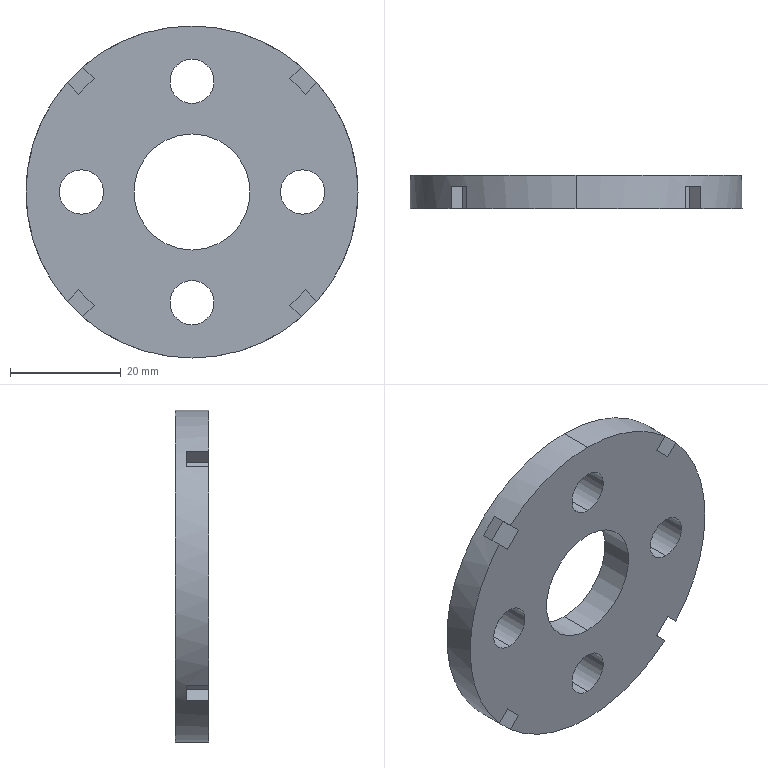Part | STEP file | Guide wheel mechanism revised.sldasm-Part-426 | 1 solid | 30 faces | box 60 x 6 x 60 mm | volume 13489 mm3 | plane 18 | cylinder 12 | commonest cylinder face diameters 8 x8 21 x2 60 x2
STEP:
#1=CARTESIAN_POINT('',(-20.,0.,4.));
#2=VERTEX_POINT('',#1);
#3=CARTESIAN_POINT('',(-20.,0.,-4.));
#4=VERTEX_POINT('',#3);
#5=CARTESIAN_POINT('',(-20.,0.,0.));
#6=DIRECTION('',(0.,-1.,0.));
#7=DIRECTION('',(0.,0.,1.));
#8=AXIS2_PLACEMENT_3D('',#5,#6,#7);
#9=CIRCLE('',#8,4.);
#10=EDGE_CURVE('',#2,#4,#9,.T.);
#11=ORIENTED_EDGE('',*,*,#10,.T.);
#12=CARTESIAN_POINT('',(-20.,6.,-4.));
#13=VERTEX_POINT('',#12);
#14=CARTESIAN_POINT('',(-20.,-0.001,-4.));
#15=DIRECTION('',(0.,1.,0.));
#16=VECTOR('',#15,1000.);
#17=LINE('',#14,#16);
#18=EDGE_CURVE('',#4,#13,#17,.T.);
#19=ORIENTED_EDGE('',*,*,#18,.T.);
#20=CARTESIAN_POINT('',(-20.,6.,4.));
#21=VERTEX_POINT('',#20);
#22=CARTESIAN_POINT('',(-20.,6.,0.));
#23=DIRECTION('',(0.,1.,0.));
#24=DIRECTION('',(0.,0.,1.));
#25=AXIS2_PLACEMENT_3D('',#22,#23,#24);
#26=CIRCLE('',#25,4.);
#27=EDGE_CURVE('',#13,#21,#26,.T.);
#28=ORIENTED_EDGE('',*,*,#27,.T.);
#29=CARTESIAN_POINT('',(-20.,-0.001,4.));
#30=DIRECTION('',(0.,1.,0.));
#31=VECTOR('',#30,1000.);
#32=LINE('',#29,#31);
#33=EDGE_CURVE('',#2,#21,#32,.T.);
#34=ORIENTED_EDGE('',*,*,#33,.F.);
#35=EDGE_LOOP('',(#11,#19,#28,#34));
#36=FACE_OUTER_BOUND('',#35,.T.);
#37=CARTESIAN_POINT('',(-20.,-0.001,0.));
#38=DIRECTION('',(0.,1.,0.));
#39=DIRECTION('',(0.,0.,1.));
#40=AXIS2_PLACEMENT_3D('',#37,#38,#39);
#41=CYLINDRICAL_SURFACE('',#40,4.);
#42=ADVANCED_FACE('',(#36),#41,.F.);
#43=CARTESIAN_POINT('',(0.,0.,24.));
#44=VERTEX_POINT('',#43);
#45=CARTESIAN_POINT('',(0.,0.,16.));
#46=VERTEX_POINT('',#45);
#47=CARTESIAN_POINT('',(0.,0.,20.));
#48=DIRECTION('',(0.,-1.,0.));
#49=DIRECTION('',(0.,0.,1.));
#50=AXIS2_PLACEMENT_3D('',#47,#48,#49);
#51=CIRCLE('',#50,4.);
#52=EDGE_CURVE('',#44,#46,#51,.T.);
#53=ORIENTED_EDGE('',*,*,#52,.T.);
#54=CARTESIAN_POINT('',(0.,6.,16.));
#55=VERTEX_POINT('',#54);
#56=CARTESIAN_POINT('',(0.,-0.001,16.));
#57=DIRECTION('',(0.,1.,0.));
#58=VECTOR('',#57,1000.);
#59=LINE('',#56,#58);
#60=EDGE_CURVE('',#46,#55,#59,.T.);
#61=ORIENTED_EDGE('',*,*,#60,.T.);
#62=CARTESIAN_POINT('',(0.,6.,24.));
#63=VERTEX_POINT('',#62);
#64=CARTESIAN_POINT('',(0.,6.,20.));
#65=DIRECTION('',(0.,1.,0.));
#66=DIRECTION('',(0.,0.,1.));
#67=AXIS2_PLACEMENT_3D('',#64,#65,#66);
#68=CIRCLE('',#67,4.);
#69=EDGE_CURVE('',#55,#63,#68,.T.);
#70=ORIENTED_EDGE('',*,*,#69,.T.);
#71=CARTESIAN_POINT('',(0.,-0.001,24.));
#72=DIRECTION('',(0.,1.,0.));
#73=VECTOR('',#72,1000.);
#74=LINE('',#71,#73);
#75=EDGE_CURVE('',#44,#63,#74,.T.);
#76=ORIENTED_EDGE('',*,*,#75,.F.);
#77=EDGE_LOOP('',(#53,#61,#70,#76));
#78=FACE_OUTER_BOUND('',#77,.T.);
#79=CARTESIAN_POINT('',(0.,-0.001,20.));
#80=DIRECTION('',(0.,1.,0.));
#81=DIRECTION('',(0.,0.,1.));
#82=AXIS2_PLACEMENT_3D('',#79,#80,#81);
#83=CYLINDRICAL_SURFACE('',#82,4.);
#84=ADVANCED_FACE('',(#78),#83,.F.);
#85=CARTESIAN_POINT('',(20.,0.,4.));
#86=VERTEX_POINT('',#85);
#87=CARTESIAN_POINT('',(20.,0.,-4.));
#88=VERTEX_POINT('',#87);
#89=CARTESIAN_POINT('',(20.,0.,0.));
#90=DIRECTION('',(0.,-1.,0.));
#91=DIRECTION('',(0.,0.,1.));
#92=AXIS2_PLACEMENT_3D('',#89,#90,#91);
#93=CIRCLE('',#92,4.);
#94=EDGE_CURVE('',#86,#88,#93,.T.);
#95=ORIENTED_EDGE('',*,*,#94,.T.);
#96=CARTESIAN_POINT('',(20.,6.,-4.));
#97=VERTEX_POINT('',#96);
#98=CARTESIAN_POINT('',(20.,-0.001,-4.));
#99=DIRECTION('',(0.,1.,0.));
#100=VECTOR('',#99,1000.);
#101=LINE('',#98,#100);
#102=EDGE_CURVE('',#88,#97,#101,.T.);
#103=ORIENTED_EDGE('',*,*,#102,.T.);
#104=CARTESIAN_POINT('',(20.,6.,4.));
#105=VERTEX_POINT('',#104);
#106=CARTESIAN_POINT('',(20.,6.,0.));
#107=DIRECTION('',(0.,1.,0.));
#108=DIRECTION('',(0.,0.,1.));
#109=AXIS2_PLACEMENT_3D('',#106,#107,#108);
#110=CIRCLE('',#109,4.);
#111=EDGE_CURVE('',#97,#105,#110,.T.);
#112=ORIENTED_EDGE('',*,*,#111,.T.);
#113=CARTESIAN_POINT('',(20.,-0.001,4.));
#114=DIRECTION('',(0.,1.,0.));
#115=VECTOR('',#114,1000.);
#116=LINE('',#113,#115);
#117=EDGE_CURVE('',#86,#105,#116,.T.);
#118=ORIENTED_EDGE('',*,*,#117,.F.);
#119=EDGE_LOOP('',(#95,#103,#112,#118));
#120=FACE_OUTER_BOUND('',#119,.T.);
#121=CARTESIAN_POINT('',(20.,-0.001,0.));
#122=DIRECTION('',(0.,1.,0.));
#123=DIRECTION('',(0.,0.,1.));
#124=AXIS2_PLACEMENT_3D('',#121,#122,#123);
#125=CYLINDRICAL_SURFACE('',#124,4.);
#126=ADVANCED_FACE('',(#120),#125,.F.);
#127=CARTESIAN_POINT('',(0.,0.,-16.));
#128=VERTEX_POINT('',#127);
#129=CARTESIAN_POINT('',(0.,0.,-24.));
#130=VERTEX_POINT('',#129);
#131=CARTESIAN_POINT('',(0.,0.,-20.));
#132=DIRECTION('',(0.,-1.,0.));
#133=DIRECTION('',(0.,0.,1.));
#134=AXIS2_PLACEMENT_3D('',#131,#132,#133);
#135=CIRCLE('',#134,4.);
#136=EDGE_CURVE('',#128,#130,#135,.T.);
#137=ORIENTED_EDGE('',*,*,#136,.T.);
#138=CARTESIAN_POINT('',(0.,6.,-24.));
#139=VERTEX_POINT('',#138);
#140=CARTESIAN_POINT('',(0.,-0.001,-24.));
#141=DIRECTION('',(0.,1.,0.));
#142=VECTOR('',#141,1000.);
#143=LINE('',#140,#142);
#144=EDGE_CURVE('',#130,#139,#143,.T.);
#145=ORIENTED_EDGE('',*,*,#144,.T.);
#146=CARTESIAN_POINT('',(0.,6.,-16.));
#147=VERTEX_POINT('',#146);
#148=CARTESIAN_POINT('',(0.,6.,-20.));
#149=DIRECTION('',(0.,1.,0.));
#150=DIRECTION('',(0.,0.,1.));
#151=AXIS2_PLACEMENT_3D('',#148,#149,#150);
#152=CIRCLE('',#151,4.);
#153=EDGE_CURVE('',#139,#147,#152,.T.);
#154=ORIENTED_EDGE('',*,*,#153,.T.);
#155=CARTESIAN_POINT('',(0.,-0.001,-16.));
#156=DIRECTION('',(0.,1.,0.));
#157=VECTOR('',#156,1000.);
#158=LINE('',#155,#157);
#159=EDGE_CURVE('',#128,#147,#158,.T.);
#160=ORIENTED_EDGE('',*,*,#159,.F.);
#161=EDGE_LOOP('',(#137,#145,#154,#160));
#162=FACE_OUTER_BOUND('',#161,.T.);
#163=CARTESIAN_POINT('',(0.,-0.001,-20.));
#164=DIRECTION('',(0.,1.,0.));
#165=DIRECTION('',(0.,0.,1.));
#166=AXIS2_PLACEMENT_3D('',#163,#164,#165);
#167=CYLINDRICAL_SURFACE('',#166,4.);
#168=ADVANCED_FACE('',(#162),#167,.F.);
#169=CARTESIAN_POINT('',(0.,6.,-10.5));
#170=VERTEX_POINT('',#169);
#171=CARTESIAN_POINT('',(0.,6.,10.5));
#172=VERTEX_POINT('',#171);
#173=CARTESIAN_POINT('',(0.,6.,0.));
#174=DIRECTION('',(0.,1.,0.));
#175=DIRECTION('',(0.,0.,1.));
#176=AXIS2_PLACEMENT_3D('',#173,#174,#175);
#177=CIRCLE('',#176,10.5);
#178=EDGE_CURVE('',#170,#172,#177,.T.);
#179=ORIENTED_EDGE('',*,*,#178,.T.);
#180=CARTESIAN_POINT('',(0.,0.,10.5));
#181=VERTEX_POINT('',#180);
#182=CARTESIAN_POINT('',(0.,6.,10.5));
#183=DIRECTION('',(0.,-1.,0.));
#184=VECTOR('',#183,1000.);
#185=LINE('',#182,#184);
#186=EDGE_CURVE('',#172,#181,#185,.T.);
#187=ORIENTED_EDGE('',*,*,#186,.T.);
#188=CARTESIAN_POINT('',(0.,0.,-10.5));
#189=VERTEX_POINT('',#188);
#190=CARTESIAN_POINT('',(0.,0.,0.));
#191=DIRECTION('',(0.,1.,0.));
#192=DIRECTION('',(0.,0.,1.));
#193=AXIS2_PLACEMENT_3D('',#190,#191,#192);
#194=CIRCLE('',#193,10.5);
#195=EDGE_CURVE('',#189,#181,#194,.T.);
#196=ORIENTED_EDGE('',*,*,#195,.F.);
#197=CARTESIAN_POINT('',(0.,6.,-10.5));
#198=DIRECTION('',(0.,-1.,0.));
#199=VECTOR('',#198,1000.);
#200=LINE('',#197,#199);
#201=EDGE_CURVE('',#170,#189,#200,.T.);
#202=ORIENTED_EDGE('',*,*,#201,.F.);
#203=EDGE_LOOP('',(#179,#187,#196,#202));
#204=FACE_OUTER_BOUND('',#203,.T.);
#205=CARTESIAN_POINT('',(0.,6.,0.));
#206=DIRECTION('',(0.,-1.,0.));
#207=DIRECTION('',(0.,0.,-1.));
#208=AXIS2_PLACEMENT_3D('',#205,#206,#207);
#209=CYLINDRICAL_SURFACE('',#208,10.5);
#210=ADVANCED_FACE('',(#204),#209,.F.);
#211=CARTESIAN_POINT('',(0.,6.,30.));
#212=VERTEX_POINT('',#211);
#213=CARTESIAN_POINT('',(0.,6.,-30.));
#214=VERTEX_POINT('',#213);
#215=CARTESIAN_POINT('',(0.,6.,0.));
#216=DIRECTION('',(0.,1.,0.));
#217=DIRECTION('',(0.,0.,1.));
#218=AXIS2_PLACEMENT_3D('',#215,#216,#217);
#219=CIRCLE('',#218,30.);
#220=EDGE_CURVE('',#212,#214,#219,.T.);
#221=ORIENTED_EDGE('',*,*,#220,.F.);
#222=CARTESIAN_POINT('',(0.,0.,30.));
#223=VERTEX_POINT('',#222);
#224=CARTESIAN_POINT('',(0.,6.,30.));
#225=DIRECTION('',(0.,-1.,0.));
#226=VECTOR('',#225,1000.);
#227=LINE('',#224,#226);
#228=EDGE_CURVE('',#212,#223,#227,.T.);
#229=ORIENTED_EDGE('',*,*,#228,.T.);
#230=CARTESIAN_POINT('',(19.752,0.,22.58));
#231=VERTEX_POINT('',#230);
#232=CARTESIAN_POINT('',(0.,0.,0.));
#233=DIRECTION('',(0.,1.,0.));
#234=DIRECTION('',(0.,0.,1.));
#235=AXIS2_PLACEMENT_3D('',#232,#233,#234);
#236=CIRCLE('',#235,30.);
#237=EDGE_CURVE('',#223,#231,#236,.T.);
#238=ORIENTED_EDGE('',*,*,#237,.T.);
#239=CARTESIAN_POINT('',(19.752,4.,22.58));
#240=VERTEX_POINT('',#239);
#241=CARTESIAN_POINT('',(19.752,4.,22.58));
#242=DIRECTION('',(0.,-1.,0.));
#243=VECTOR('',#242,1000.);
#244=LINE('',#241,#243);
#245=EDGE_CURVE('',#240,#231,#244,.T.);
#246=ORIENTED_EDGE('',*,*,#245,.F.);
#247=CARTESIAN_POINT('',(22.58,4.,19.752));
#248=VERTEX_POINT('',#247);
#249=CARTESIAN_POINT('',(0.,4.,0.));
#250=DIRECTION('',(0.,-1.,0.));
#251=DIRECTION('',(0.,0.,-1.));
#252=AXIS2_PLACEMENT_3D('',#249,#250,#251);
#253=CIRCLE('',#252,30.);
#254=EDGE_CURVE('',#248,#240,#253,.T.);
#255=ORIENTED_EDGE('',*,*,#254,.F.);
#256=CARTESIAN_POINT('',(22.58,0.,19.752));
#257=VERTEX_POINT('',#256);
#258=CARTESIAN_POINT('',(22.58,4.,19.752));
#259=DIRECTION('',(0.,-1.,0.));
#260=VECTOR('',#259,1000.);
#261=LINE('',#258,#260);
#262=EDGE_CURVE('',#248,#257,#261,.T.);
#263=ORIENTED_EDGE('',*,*,#262,.T.);
#264=CARTESIAN_POINT('',(22.58,0.,-19.752));
#265=VERTEX_POINT('',#264);
#266=CARTESIAN_POINT('',(0.,0.,0.));
#267=DIRECTION('',(0.,1.,0.));
#268=DIRECTION('',(0.,0.,1.));
#269=AXIS2_PLACEMENT_3D('',#266,#267,#268);
#270=CIRCLE('',#269,30.);
#271=EDGE_CURVE('',#257,#265,#270,.T.);
#272=ORIENTED_EDGE('',*,*,#271,.T.);
#273=CARTESIAN_POINT('',(22.58,4.,-19.752));
#274=VERTEX_POINT('',#273);
#275=CARTESIAN_POINT('',(22.58,4.,-19.752));
#276=DIRECTION('',(0.,-1.,0.));
#277=VECTOR('',#276,1000.);
#278=LINE('',#275,#277);
#279=EDGE_CURVE('',#274,#265,#278,.T.);
#280=ORIENTED_EDGE('',*,*,#279,.F.);
#281=CARTESIAN_POINT('',(19.752,4.,-22.58));
#282=VERTEX_POINT('',#281);
#283=CARTESIAN_POINT('',(0.,4.,0.));
#284=DIRECTION('',(0.,-1.,0.));
#285=DIRECTION('',(0.,0.,-1.));
#286=AXIS2_PLACEMENT_3D('',#283,#284,#285);
#287=CIRCLE('',#286,30.);
#288=EDGE_CURVE('',#282,#274,#287,.T.);
#289=ORIENTED_EDGE('',*,*,#288,.F.);
#290=CARTESIAN_POINT('',(19.752,0.,-22.58));
#291=VERTEX_POINT('',#290);
#292=CARTESIAN_POINT('',(19.752,4.,-22.58));
#293=DIRECTION('',(0.,-1.,0.));
#294=VECTOR('',#293,1000.);
#295=LINE('',#292,#294);
#296=EDGE_CURVE('',#282,#291,#295,.T.);
#297=ORIENTED_EDGE('',*,*,#296,.T.);
#298=CARTESIAN_POINT('',(0.,0.,-30.));
#299=VERTEX_POINT('',#298);
#300=CARTESIAN_POINT('',(0.,0.,0.));
#301=DIRECTION('',(0.,1.,0.));
#302=DIRECTION('',(0.,0.,1.));
#303=AXIS2_PLACEMENT_3D('',#300,#301,#302);
#304=CIRCLE('',#303,30.);
#305=EDGE_CURVE('',#291,#299,#304,.T.);
#306=ORIENTED_EDGE('',*,*,#305,.T.);
#307=CARTESIAN_POINT('',(0.,6.,-30.));
#308=DIRECTION('',(0.,-1.,0.));
#309=VECTOR('',#308,1000.);
#310=LINE('',#307,#309);
#311=EDGE_CURVE('',#214,#299,#310,.T.);
#312=ORIENTED_EDGE('',*,*,#311,.F.);
#313=EDGE_LOOP('',(#221,#229,#238,#246,#255,#263,#272,#280,#289,#297,#306,#312));
#314=FACE_OUTER_BOUND('',#313,.T.);
#315=CARTESIAN_POINT('',(0.,6.,0.));
#316=DIRECTION('',(0.,-1.,0.));
#317=DIRECTION('',(0.,0.,-1.));
#318=AXIS2_PLACEMENT_3D('',#315,#316,#317);
#319=CYLINDRICAL_SURFACE('',#318,30.);
#320=ADVANCED_FACE('',(#314),#319,.T.);
#321=CARTESIAN_POINT('',(-20.,6.,0.));
#322=DIRECTION('',(0.,1.,0.));
#323=DIRECTION('',(0.,0.,1.));
#324=AXIS2_PLACEMENT_3D('',#321,#322,#323);
#325=CIRCLE('',#324,4.);
#326=EDGE_CURVE('',#21,#13,#325,.T.);
#327=ORIENTED_EDGE('',*,*,#326,.F.);
#328=ORIENTED_EDGE('',*,*,#27,.F.);
#329=EDGE_LOOP('',(#327,#328));
#330=FACE_BOUND('',#329,.T.);
#331=CARTESIAN_POINT('',(0.,6.,20.));
#332=DIRECTION('',(0.,1.,0.));
#333=DIRECTION('',(0.,0.,1.));
#334=AXIS2_PLACEMENT_3D('',#331,#332,#333);
#335=CIRCLE('',#334,4.);
#336=EDGE_CURVE('',#63,#55,#335,.T.);
#337=ORIENTED_EDGE('',*,*,#336,.F.);
#338=ORIENTED_EDGE('',*,*,#69,.F.);
#339=EDGE_LOOP('',(#337,#338));
#340=FACE_BOUND('',#339,.T.);
#341=CARTESIAN_POINT('',(20.,6.,0.));
#342=DIRECTION('',(0.,1.,0.));
#343=DIRECTION('',(0.,0.,1.));
#344=AXIS2_PLACEMENT_3D('',#341,#342,#343);
#345=CIRCLE('',#344,4.);
#346=EDGE_CURVE('',#105,#97,#345,.T.);
#347=ORIENTED_EDGE('',*,*,#346,.F.);
#348=ORIENTED_EDGE('',*,*,#111,.F.);
#349=EDGE_LOOP('',(#347,#348));
#350=FACE_BOUND('',#349,.T.);
#351=CARTESIAN_POINT('',(0.,6.,-20.));
#352=DIRECTION('',(0.,1.,0.));
#353=DIRECTION('',(0.,0.,1.));
#354=AXIS2_PLACEMENT_3D('',#351,#352,#353);
#355=CIRCLE('',#354,4.);
#356=EDGE_CURVE('',#147,#139,#355,.T.);
#357=ORIENTED_EDGE('',*,*,#356,.F.);
#358=ORIENTED_EDGE('',*,*,#153,.F.);
#359=EDGE_LOOP('',(#357,#358));
#360=FACE_BOUND('',#359,.T.);
#361=CARTESIAN_POINT('',(0.,6.,0.));
#362=DIRECTION('',(0.,1.,0.));
#363=DIRECTION('',(0.,0.,1.));
#364=AXIS2_PLACEMENT_3D('',#361,#362,#363);
#365=CIRCLE('',#364,30.);
#366=EDGE_CURVE('',#214,#212,#365,.T.);
#367=ORIENTED_EDGE('',*,*,#366,.T.);
#368=ORIENTED_EDGE('',*,*,#220,.T.);
#369=EDGE_LOOP('',(#367,#368));
#370=FACE_OUTER_BOUND('',#369,.T.);
#371=ORIENTED_EDGE('',*,*,#178,.F.);
#372=CARTESIAN_POINT('',(0.,6.,0.));
#373=DIRECTION('',(0.,1.,0.));
#374=DIRECTION('',(0.,0.,1.));
#375=AXIS2_PLACEMENT_3D('',#372,#373,#374);
#376=CIRCLE('',#375,10.5);
#377=EDGE_CURVE('',#172,#170,#376,.T.);
#378=ORIENTED_EDGE('',*,*,#377,.F.);
#379=EDGE_LOOP('',(#371,#378));
#380=FACE_BOUND('',#379,.T.);
#381=CARTESIAN_POINT('',(0.,6.,0.));
#382=DIRECTION('',(0.,1.,0.));
#383=DIRECTION('',(0.,0.,1.));
#384=AXIS2_PLACEMENT_3D('',#381,#382,#383);
#385=PLANE('',#384);
#386=ADVANCED_FACE('',(#330,#340,#350,#360,#370,#380),#385,.T.);
#387=ORIENTED_EDGE('',*,*,#10,.F.);
#388=CARTESIAN_POINT('',(-20.,0.,0.));
#389=DIRECTION('',(0.,-1.,0.));
#390=DIRECTION('',(0.,0.,1.));
#391=AXIS2_PLACEMENT_3D('',#388,#389,#390);
#392=CIRCLE('',#391,4.);
#393=EDGE_CURVE('',#4,#2,#392,.T.);
#394=ORIENTED_EDGE('',*,*,#393,.F.);
#395=EDGE_LOOP('',(#387,#394));
#396=FACE_BOUND('',#395,.T.);
#397=ORIENTED_EDGE('',*,*,#52,.F.);
#398=CARTESIAN_POINT('',(0.,0.,20.));
#399=DIRECTION('',(0.,-1.,0.));
#400=DIRECTION('',(0.,0.,1.));
#401=AXIS2_PLACEMENT_3D('',#398,#399,#400);
#402=CIRCLE('',#401,4.);
#403=EDGE_CURVE('',#46,#44,#402,.T.);
#404=ORIENTED_EDGE('',*,*,#403,.F.);
#405=EDGE_LOOP('',(#397,#404));
#406=FACE_BOUND('',#405,.T.);
#407=ORIENTED_EDGE('',*,*,#94,.F.);
#408=CARTESIAN_POINT('',(20.,0.,0.));
#409=DIRECTION('',(0.,-1.,0.));
#410=DIRECTION('',(0.,0.,1.));
#411=AXIS2_PLACEMENT_3D('',#408,#409,#410);
#412=CIRCLE('',#411,4.);
#413=EDGE_CURVE('',#88,#86,#412,.T.);
#414=ORIENTED_EDGE('',*,*,#413,.F.);
#415=EDGE_LOOP('',(#407,#414));
#416=FACE_BOUND('',#415,.T.);
#417=ORIENTED_EDGE('',*,*,#136,.F.);
#418=CARTESIAN_POINT('',(0.,0.,-20.));
#419=DIRECTION('',(0.,-1.,0.));
#420=DIRECTION('',(0.,0.,1.));
#421=AXIS2_PLACEMENT_3D('',#418,#419,#420);
#422=CIRCLE('',#421,4.);
#423=EDGE_CURVE('',#130,#128,#422,.T.);
#424=ORIENTED_EDGE('',*,*,#423,.F.);
#425=EDGE_LOOP('',(#417,#424));
#426=FACE_BOUND('',#425,.T.);
#427=CARTESIAN_POINT('',(-17.678,0.,-20.506));
#428=VERTEX_POINT('',#427);
#429=CARTESIAN_POINT('',(-20.506,0.,-17.678));
#430=VERTEX_POINT('',#429);
#431=CARTESIAN_POINT('',(-17.678,0.,-20.506));
#432=DIRECTION('',(-0.7071,0.,0.7071));
#433=VECTOR('',#432,1000.);
#434=LINE('',#431,#433);
#435=EDGE_CURVE('',#428,#430,#434,.T.);
#436=ORIENTED_EDGE('',*,*,#435,.F.);
#437=CARTESIAN_POINT('',(-19.752,0.,-22.58));
#438=VERTEX_POINT('',#437);
#439=CARTESIAN_POINT('',(-17.678,0.,-20.506));
#440=DIRECTION('',(0.7071,0.,0.7071));
#441=VECTOR('',#440,1000.);
#442=LINE('',#439,#441);
#443=EDGE_CURVE('',#438,#428,#442,.T.);
#444=ORIENTED_EDGE('',*,*,#443,.F.);
#445=CARTESIAN_POINT('',(0.,0.,0.));
#446=DIRECTION('',(0.,1.,0.));
#447=DIRECTION('',(0.,0.,1.));
#448=AXIS2_PLACEMENT_3D('',#445,#446,#447);
#449=CIRCLE('',#448,30.);
#450=EDGE_CURVE('',#299,#438,#449,.T.);
#451=ORIENTED_EDGE('',*,*,#450,.F.);
#452=ORIENTED_EDGE('',*,*,#305,.F.);
#453=CARTESIAN_POINT('',(17.678,0.,-20.506));
#454=VERTEX_POINT('',#453);
#455=CARTESIAN_POINT('',(17.678,0.,-20.506));
#456=DIRECTION('',(0.7071,0.,-0.7071));
#457=VECTOR('',#456,1000.);
#458=LINE('',#455,#457);
#459=EDGE_CURVE('',#454,#291,#458,.T.);
#460=ORIENTED_EDGE('',*,*,#459,.F.);
#461=CARTESIAN_POINT('',(20.506,0.,-17.678));
#462=VERTEX_POINT('',#461);
#463=CARTESIAN_POINT('',(20.506,0.,-17.678));
#464=DIRECTION('',(-0.7071,0.,-0.7071));
#465=VECTOR('',#464,1000.);
#466=LINE('',#463,#465);
#467=EDGE_CURVE('',#462,#454,#466,.T.);
#468=ORIENTED_EDGE('',*,*,#467,.F.);
#469=CARTESIAN_POINT('',(20.506,0.,-17.678));
#470=DIRECTION('',(-0.7071,0.,0.7071));
#471=VECTOR('',#470,1000.);
#472=LINE('',#469,#471);
#473=EDGE_CURVE('',#265,#462,#472,.T.);
#474=ORIENTED_EDGE('',*,*,#473,.F.);
#475=ORIENTED_EDGE('',*,*,#271,.F.);
#476=CARTESIAN_POINT('',(20.506,0.,17.678));
#477=VERTEX_POINT('',#476);
#478=CARTESIAN_POINT('',(22.58,0.,19.752));
#479=DIRECTION('',(0.7071,0.,0.7071));
#480=VECTOR('',#479,1000.);
#481=LINE('',#478,#480);
#482=EDGE_CURVE('',#477,#257,#481,.T.);
#483=ORIENTED_EDGE('',*,*,#482,.F.);
#484=CARTESIAN_POINT('',(17.678,0.,20.506));
#485=VERTEX_POINT('',#484);
#486=CARTESIAN_POINT('',(17.678,0.,20.506));
#487=DIRECTION('',(0.7071,0.,-0.7071));
#488=VECTOR('',#487,1000.);
#489=LINE('',#486,#488);
#490=EDGE_CURVE('',#485,#477,#489,.T.);
#491=ORIENTED_EDGE('',*,*,#490,.F.);
#492=CARTESIAN_POINT('',(19.752,0.,22.58));
#493=DIRECTION('',(-0.7071,0.,-0.7071));
#494=VECTOR('',#493,1000.);
#495=LINE('',#492,#494);
#496=EDGE_CURVE('',#231,#485,#495,.T.);
#497=ORIENTED_EDGE('',*,*,#496,.F.);
#498=ORIENTED_EDGE('',*,*,#237,.F.);
#499=CARTESIAN_POINT('',(-19.752,0.,22.58));
#500=VERTEX_POINT('',#499);
#501=CARTESIAN_POINT('',(0.,0.,0.));
#502=DIRECTION('',(0.,1.,0.));
#503=DIRECTION('',(0.,0.,1.));
#504=AXIS2_PLACEMENT_3D('',#501,#502,#503);
#505=CIRCLE('',#504,30.);
#506=EDGE_CURVE('',#500,#223,#505,.T.);
#507=ORIENTED_EDGE('',*,*,#506,.F.);
#508=CARTESIAN_POINT('',(-17.678,0.,20.506));
#509=VERTEX_POINT('',#508);
#510=CARTESIAN_POINT('',(-19.752,0.,22.58));
#511=DIRECTION('',(-0.7071,0.,0.7071));
#512=VECTOR('',#511,1000.);
#513=LINE('',#510,#512);
#514=EDGE_CURVE('',#509,#500,#513,.T.);
#515=ORIENTED_EDGE('',*,*,#514,.F.);
#516=CARTESIAN_POINT('',(-20.506,0.,17.678));
#517=VERTEX_POINT('',#516);
#518=CARTESIAN_POINT('',(-17.678,0.,20.506));
#519=DIRECTION('',(0.7071,0.,0.7071));
#520=VECTOR('',#519,1000.);
#521=LINE('',#518,#520);
#522=EDGE_CURVE('',#517,#509,#521,.T.);
#523=ORIENTED_EDGE('',*,*,#522,.F.);
#524=CARTESIAN_POINT('',(-22.58,0.,19.752));
#525=VERTEX_POINT('',#524);
#526=CARTESIAN_POINT('',(-22.58,0.,19.752));
#527=DIRECTION('',(0.7071,0.,-0.7071));
#528=VECTOR('',#527,1000.);
#529=LINE('',#526,#528);
#530=EDGE_CURVE('',#525,#517,#529,.T.);
#531=ORIENTED_EDGE('',*,*,#530,.F.);
#532=CARTESIAN_POINT('',(-22.58,0.,-19.752));
#533=VERTEX_POINT('',#532);
#534=CARTESIAN_POINT('',(0.,0.,0.));
#535=DIRECTION('',(0.,1.,0.));
#536=DIRECTION('',(0.,0.,1.));
#537=AXIS2_PLACEMENT_3D('',#534,#535,#536);
#538=CIRCLE('',#537,30.);
#539=EDGE_CURVE('',#533,#525,#538,.T.);
#540=ORIENTED_EDGE('',*,*,#539,.F.);
#541=CARTESIAN_POINT('',(-20.506,0.,-17.678));
#542=DIRECTION('',(-0.7071,0.,-0.7071));
#543=VECTOR('',#542,1000.);
#544=LINE('',#541,#543);
#545=EDGE_CURVE('',#430,#533,#544,.T.);
#546=ORIENTED_EDGE('',*,*,#545,.F.);
#547=EDGE_LOOP('',(#436,#444,#451,#452,#460,#468,#474,#475,#483,#491,#497,#498,#507,#515,#523,#531,#540,#546));
#548=FACE_OUTER_BOUND('',#547,.T.);
#549=ORIENTED_EDGE('',*,*,#195,.T.);
#550=CARTESIAN_POINT('',(0.,0.,0.));
#551=DIRECTION('',(0.,1.,0.));
#552=DIRECTION('',(0.,0.,1.));
#553=AXIS2_PLACEMENT_3D('',#550,#551,#552);
#554=CIRCLE('',#553,10.5);
#555=EDGE_CURVE('',#181,#189,#554,.T.);
#556=ORIENTED_EDGE('',*,*,#555,.T.);
#557=EDGE_LOOP('',(#549,#556));
#558=FACE_BOUND('',#557,.T.);
#559=CARTESIAN_POINT('',(0.,0.,0.));
#560=DIRECTION('',(0.,1.,0.));
#561=DIRECTION('',(0.,0.,1.));
#562=AXIS2_PLACEMENT_3D('',#559,#560,#561);
#563=PLANE('',#562);
#564=ADVANCED_FACE('',(#396,#406,#416,#426,#548,#558),#563,.F.);
#565=ORIENTED_EDGE('',*,*,#228,.F.);
#566=ORIENTED_EDGE('',*,*,#366,.F.);
#567=ORIENTED_EDGE('',*,*,#311,.T.);
#568=ORIENTED_EDGE('',*,*,#450,.T.);
#569=CARTESIAN_POINT('',(-19.752,4.,-22.58));
#570=VERTEX_POINT('',#569);
#571=CARTESIAN_POINT('',(-19.752,4.,-22.58));
#572=DIRECTION('',(0.,-1.,0.));
#573=VECTOR('',#572,1000.);
#574=LINE('',#571,#573);
#575=EDGE_CURVE('',#570,#438,#574,.T.);
#576=ORIENTED_EDGE('',*,*,#575,.F.);
#577=CARTESIAN_POINT('',(-22.58,4.,-19.752));
#578=VERTEX_POINT('',#577);
#579=CARTESIAN_POINT('',(0.,4.,0.));
#580=DIRECTION('',(0.,-1.,0.));
#581=DIRECTION('',(0.,0.,-1.));
#582=AXIS2_PLACEMENT_3D('',#579,#580,#581);
#583=CIRCLE('',#582,30.);
#584=EDGE_CURVE('',#578,#570,#583,.T.);
#585=ORIENTED_EDGE('',*,*,#584,.F.);
#586=CARTESIAN_POINT('',(-22.58,4.,-19.752));
#587=DIRECTION('',(0.,-1.,0.));
#588=VECTOR('',#587,1000.);
#589=LINE('',#586,#588);
#590=EDGE_CURVE('',#578,#533,#589,.T.);
#591=ORIENTED_EDGE('',*,*,#590,.T.);
#592=ORIENTED_EDGE('',*,*,#539,.T.);
#593=CARTESIAN_POINT('',(-22.58,4.,19.752));
#594=VERTEX_POINT('',#593);
#595=CARTESIAN_POINT('',(-22.58,4.,19.752));
#596=DIRECTION('',(0.,-1.,0.));
#597=VECTOR('',#596,1000.);
#598=LINE('',#595,#597);
#599=EDGE_CURVE('',#594,#525,#598,.T.);
#600=ORIENTED_EDGE('',*,*,#599,.F.);
#601=CARTESIAN_POINT('',(-19.752,4.,22.58));
#602=VERTEX_POINT('',#601);
#603=CARTESIAN_POINT('',(0.,4.,0.));
#604=DIRECTION('',(0.,-1.,0.));
#605=DIRECTION('',(0.,0.,-1.));
#606=AXIS2_PLACEMENT_3D('',#603,#604,#605);
#607=CIRCLE('',#606,30.);
#608=EDGE_CURVE('',#602,#594,#607,.T.);
#609=ORIENTED_EDGE('',*,*,#608,.F.);
#610=CARTESIAN_POINT('',(-19.752,4.,22.58));
#611=DIRECTION('',(0.,-1.,0.));
#612=VECTOR('',#611,1000.);
#613=LINE('',#610,#612);
#614=EDGE_CURVE('',#602,#500,#613,.T.);
#615=ORIENTED_EDGE('',*,*,#614,.T.);
#616=ORIENTED_EDGE('',*,*,#506,.T.);
#617=EDGE_LOOP('',(#565,#566,#567,#568,#576,#585,#591,#592,#600,#609,#615,#616));
#618=FACE_OUTER_BOUND('',#617,.T.);
#619=CARTESIAN_POINT('',(0.,6.,0.));
#620=DIRECTION('',(0.,-1.,0.));
#621=DIRECTION('',(0.,0.,-1.));
#622=AXIS2_PLACEMENT_3D('',#619,#620,#621);
#623=CYLINDRICAL_SURFACE('',#622,30.);
#624=ADVANCED_FACE('',(#618),#623,.T.);
#625=ORIENTED_EDGE('',*,*,#186,.F.);
#626=ORIENTED_EDGE('',*,*,#377,.T.);
#627=ORIENTED_EDGE('',*,*,#201,.T.);
#628=ORIENTED_EDGE('',*,*,#555,.F.);
#629=EDGE_LOOP('',(#625,#626,#627,#628));
#630=FACE_OUTER_BOUND('',#629,.T.);
#631=CARTESIAN_POINT('',(0.,6.,0.));
#632=DIRECTION('',(0.,-1.,0.));
#633=DIRECTION('',(0.,0.,-1.));
#634=AXIS2_PLACEMENT_3D('',#631,#632,#633);
#635=CYLINDRICAL_SURFACE('',#634,10.5);
#636=ADVANCED_FACE('',(#630),#635,.F.);
#637=ORIENTED_EDGE('',*,*,#144,.F.);
#638=ORIENTED_EDGE('',*,*,#423,.T.);
#639=ORIENTED_EDGE('',*,*,#159,.T.);
#640=ORIENTED_EDGE('',*,*,#356,.T.);
#641=EDGE_LOOP('',(#637,#638,#639,#640));
#642=FACE_OUTER_BOUND('',#641,.T.);
#643=CARTESIAN_POINT('',(0.,-0.001,-20.));
#644=DIRECTION('',(0.,1.,0.));
#645=DIRECTION('',(0.,0.,1.));
#646=AXIS2_PLACEMENT_3D('',#643,#644,#645);
#647=CYLINDRICAL_SURFACE('',#646,4.);
#648=ADVANCED_FACE('',(#642),#647,.F.);
#649=ORIENTED_EDGE('',*,*,#102,.F.);
#650=ORIENTED_EDGE('',*,*,#413,.T.);
#651=ORIENTED_EDGE('',*,*,#117,.T.);
#652=ORIENTED_EDGE('',*,*,#346,.T.);
#653=EDGE_LOOP('',(#649,#650,#651,#652));
#654=FACE_OUTER_BOUND('',#653,.T.);
#655=CARTESIAN_POINT('',(20.,-0.001,0.));
#656=DIRECTION('',(0.,1.,0.));
#657=DIRECTION('',(0.,0.,1.));
#658=AXIS2_PLACEMENT_3D('',#655,#656,#657);
#659=CYLINDRICAL_SURFACE('',#658,4.);
#660=ADVANCED_FACE('',(#654),#659,.F.);
#661=ORIENTED_EDGE('',*,*,#60,.F.);
#662=ORIENTED_EDGE('',*,*,#403,.T.);
#663=ORIENTED_EDGE('',*,*,#75,.T.);
#664=ORIENTED_EDGE('',*,*,#336,.T.);
#665=EDGE_LOOP('',(#661,#662,#663,#664));
#666=FACE_OUTER_BOUND('',#665,.T.);
#667=CARTESIAN_POINT('',(0.,-0.001,20.));
#668=DIRECTION('',(0.,1.,0.));
#669=DIRECTION('',(0.,0.,1.));
#670=AXIS2_PLACEMENT_3D('',#667,#668,#669);
#671=CYLINDRICAL_SURFACE('',#670,4.);
#672=ADVANCED_FACE('',(#666),#671,.F.);
#673=ORIENTED_EDGE('',*,*,#18,.F.);
#674=ORIENTED_EDGE('',*,*,#393,.T.);
#675=ORIENTED_EDGE('',*,*,#33,.T.);
#676=ORIENTED_EDGE('',*,*,#326,.T.);
#677=EDGE_LOOP('',(#673,#674,#675,#676));
#678=FACE_OUTER_BOUND('',#677,.T.);
#679=CARTESIAN_POINT('',(-20.,-0.001,0.));
#680=DIRECTION('',(0.,1.,0.));
#681=DIRECTION('',(0.,0.,1.));
#682=AXIS2_PLACEMENT_3D('',#679,#680,#681);
#683=CYLINDRICAL_SURFACE('',#682,4.);
#684=ADVANCED_FACE('',(#678),#683,.F.);
#685=ORIENTED_EDGE('',*,*,#482,.T.);
#686=ORIENTED_EDGE('',*,*,#262,.F.);
#687=CARTESIAN_POINT('',(20.506,4.,17.678));
#688=VERTEX_POINT('',#687);
#689=CARTESIAN_POINT('',(22.58,4.,19.752));
#690=DIRECTION('',(0.7071,0.,0.7071));
#691=VECTOR('',#690,1000.);
#692=LINE('',#689,#691);
#693=EDGE_CURVE('',#688,#248,#692,.T.);
#694=ORIENTED_EDGE('',*,*,#693,.F.);
#695=CARTESIAN_POINT('',(20.506,4.,17.678));
#696=DIRECTION('',(0.,-1.,0.));
#697=VECTOR('',#696,1000.);
#698=LINE('',#695,#697);
#699=EDGE_CURVE('',#688,#477,#698,.T.);
#700=ORIENTED_EDGE('',*,*,#699,.T.);
#701=EDGE_LOOP('',(#685,#686,#694,#700));
#702=FACE_OUTER_BOUND('',#701,.T.);
#703=CARTESIAN_POINT('',(22.58,4.,19.752));
#704=DIRECTION('',(0.7071,0.,-0.7071));
#705=DIRECTION('',(-0.7071,0.,-0.7071));
#706=AXIS2_PLACEMENT_3D('',#703,#704,#705);
#707=PLANE('',#706);
#708=ADVANCED_FACE('',(#702),#707,.F.);
#709=ORIENTED_EDGE('',*,*,#490,.T.);
#710=ORIENTED_EDGE('',*,*,#699,.F.);
#711=CARTESIAN_POINT('',(17.678,4.,20.506));
#712=VERTEX_POINT('',#711);
#713=CARTESIAN_POINT('',(17.678,4.,20.506));
#714=DIRECTION('',(0.7071,0.,-0.7071));
#715=VECTOR('',#714,1000.);
#716=LINE('',#713,#715);
#717=EDGE_CURVE('',#712,#688,#716,.T.);
#718=ORIENTED_EDGE('',*,*,#717,.F.);
#719=CARTESIAN_POINT('',(17.678,4.,20.506));
#720=DIRECTION('',(0.,-1.,0.));
#721=VECTOR('',#720,1000.);
#722=LINE('',#719,#721);
#723=EDGE_CURVE('',#712,#485,#722,.T.);
#724=ORIENTED_EDGE('',*,*,#723,.T.);
#725=EDGE_LOOP('',(#709,#710,#718,#724));
#726=FACE_OUTER_BOUND('',#725,.T.);
#727=CARTESIAN_POINT('',(17.678,4.,20.506));
#728=DIRECTION('',(-0.7071,0.,-0.7071));
#729=DIRECTION('',(-0.7071,0.,0.7071));
#730=AXIS2_PLACEMENT_3D('',#727,#728,#729);
#731=PLANE('',#730);
#732=ADVANCED_FACE('',(#726),#731,.F.);
#733=ORIENTED_EDGE('',*,*,#496,.T.);
#734=ORIENTED_EDGE('',*,*,#723,.F.);
#735=CARTESIAN_POINT('',(19.752,4.,22.58));
#736=DIRECTION('',(-0.7071,0.,-0.7071));
#737=VECTOR('',#736,1000.);
#738=LINE('',#735,#737);
#739=EDGE_CURVE('',#240,#712,#738,.T.);
#740=ORIENTED_EDGE('',*,*,#739,.F.);
#741=ORIENTED_EDGE('',*,*,#245,.T.);
#742=EDGE_LOOP('',(#733,#734,#740,#741));
#743=FACE_OUTER_BOUND('',#742,.T.);
#744=CARTESIAN_POINT('',(19.752,4.,22.58));
#745=DIRECTION('',(-0.7071,0.,0.7071));
#746=DIRECTION('',(0.7071,0.,0.7071));
#747=AXIS2_PLACEMENT_3D('',#744,#745,#746);
#748=PLANE('',#747);
#749=ADVANCED_FACE('',(#743),#748,.F.);
#750=ORIENTED_EDGE('',*,*,#254,.T.);
#751=ORIENTED_EDGE('',*,*,#739,.T.);
#752=ORIENTED_EDGE('',*,*,#717,.T.);
#753=ORIENTED_EDGE('',*,*,#693,.T.);
#754=EDGE_LOOP('',(#750,#751,#752,#753));
#755=FACE_OUTER_BOUND('',#754,.T.);
#756=CARTESIAN_POINT('',(0.,4.,0.));
#757=DIRECTION('',(0.,-1.,0.));
#758=DIRECTION('',(0.,0.,-1.));
#759=AXIS2_PLACEMENT_3D('',#756,#757,#758);
#760=PLANE('',#759);
#761=ADVANCED_FACE('',(#755),#760,.T.);
#762=ORIENTED_EDGE('',*,*,#522,.T.);
#763=CARTESIAN_POINT('',(-17.678,4.,20.506));
#764=VERTEX_POINT('',#763);
#765=CARTESIAN_POINT('',(-17.678,4.,20.506));
#766=DIRECTION('',(0.,-1.,0.));
#767=VECTOR('',#766,1000.);
#768=LINE('',#765,#767);
#769=EDGE_CURVE('',#764,#509,#768,.T.);
#770=ORIENTED_EDGE('',*,*,#769,.F.);
#771=CARTESIAN_POINT('',(-20.506,4.,17.678));
#772=VERTEX_POINT('',#771);
#773=CARTESIAN_POINT('',(-17.678,4.,20.506));
#774=DIRECTION('',(0.7071,0.,0.7071));
#775=VECTOR('',#774,1000.);
#776=LINE('',#773,#775);
#777=EDGE_CURVE('',#772,#764,#776,.T.);
#778=ORIENTED_EDGE('',*,*,#777,.F.);
#779=CARTESIAN_POINT('',(-20.506,4.,17.678));
#780=DIRECTION('',(0.,-1.,0.));
#781=VECTOR('',#780,1000.);
#782=LINE('',#779,#781);
#783=EDGE_CURVE('',#772,#517,#782,.T.);
#784=ORIENTED_EDGE('',*,*,#783,.T.);
#785=EDGE_LOOP('',(#762,#770,#778,#784));
#786=FACE_OUTER_BOUND('',#785,.T.);
#787=CARTESIAN_POINT('',(-17.678,4.,20.506));
#788=DIRECTION('',(0.7071,0.,-0.7071));
#789=DIRECTION('',(-0.7071,0.,-0.7071));
#790=AXIS2_PLACEMENT_3D('',#787,#788,#789);
#791=PLANE('',#790);
#792=ADVANCED_FACE('',(#786),#791,.F.);
#793=ORIENTED_EDGE('',*,*,#530,.T.);
#794=ORIENTED_EDGE('',*,*,#783,.F.);
#795=CARTESIAN_POINT('',(-22.58,4.,19.752));
#796=DIRECTION('',(0.7071,0.,-0.7071));
#797=VECTOR('',#796,1000.);
#798=LINE('',#795,#797);
#799=EDGE_CURVE('',#594,#772,#798,.T.);
#800=ORIENTED_EDGE('',*,*,#799,.F.);
#801=ORIENTED_EDGE('',*,*,#599,.T.);
#802=EDGE_LOOP('',(#793,#794,#800,#801));
#803=FACE_OUTER_BOUND('',#802,.T.);
#804=CARTESIAN_POINT('',(-22.58,4.,19.752));
#805=DIRECTION('',(-0.7071,0.,-0.7071));
#806=DIRECTION('',(-0.7071,0.,0.7071));
#807=AXIS2_PLACEMENT_3D('',#804,#805,#806);
#808=PLANE('',#807);
#809=ADVANCED_FACE('',(#803),#808,.F.);
#810=ORIENTED_EDGE('',*,*,#514,.T.);
#811=ORIENTED_EDGE('',*,*,#614,.F.);
#812=CARTESIAN_POINT('',(-19.752,4.,22.58));
#813=DIRECTION('',(-0.7071,0.,0.7071));
#814=VECTOR('',#813,1000.);
#815=LINE('',#812,#814);
#816=EDGE_CURVE('',#764,#602,#815,.T.);
#817=ORIENTED_EDGE('',*,*,#816,.F.);
#818=ORIENTED_EDGE('',*,*,#769,.T.);
#819=EDGE_LOOP('',(#810,#811,#817,#818));
#820=FACE_OUTER_BOUND('',#819,.T.);
#821=CARTESIAN_POINT('',(-19.752,4.,22.58));
#822=DIRECTION('',(0.7071,0.,0.7071));
#823=DIRECTION('',(0.7071,0.,-0.7071));
#824=AXIS2_PLACEMENT_3D('',#821,#822,#823);
#825=PLANE('',#824);
#826=ADVANCED_FACE('',(#820),#825,.F.);
#827=ORIENTED_EDGE('',*,*,#777,.T.);
#828=ORIENTED_EDGE('',*,*,#816,.T.);
#829=ORIENTED_EDGE('',*,*,#608,.T.);
#830=ORIENTED_EDGE('',*,*,#799,.T.);
#831=EDGE_LOOP('',(#827,#828,#829,#830));
#832=FACE_OUTER_BOUND('',#831,.T.);
#833=CARTESIAN_POINT('',(0.,4.,0.));
#834=DIRECTION('',(0.,-1.,0.));
#835=DIRECTION('',(0.,0.,-1.));
#836=AXIS2_PLACEMENT_3D('',#833,#834,#835);
#837=PLANE('',#836);
#838=ADVANCED_FACE('',(#832),#837,.T.);
#839=ORIENTED_EDGE('',*,*,#473,.T.);
#840=CARTESIAN_POINT('',(20.506,4.,-17.678));
#841=VERTEX_POINT('',#840);
#842=CARTESIAN_POINT('',(20.506,4.,-17.678));
#843=DIRECTION('',(0.,-1.,0.));
#844=VECTOR('',#843,1000.);
#845=LINE('',#842,#844);
#846=EDGE_CURVE('',#841,#462,#845,.T.);
#847=ORIENTED_EDGE('',*,*,#846,.F.);
#848=CARTESIAN_POINT('',(20.506,4.,-17.678));
#849=DIRECTION('',(-0.7071,0.,0.7071));
#850=VECTOR('',#849,1000.);
#851=LINE('',#848,#850);
#852=EDGE_CURVE('',#274,#841,#851,.T.);
#853=ORIENTED_EDGE('',*,*,#852,.F.);
#854=ORIENTED_EDGE('',*,*,#279,.T.);
#855=EDGE_LOOP('',(#839,#847,#853,#854));
#856=FACE_OUTER_BOUND('',#855,.T.);
#857=CARTESIAN_POINT('',(20.506,4.,-17.678));
#858=DIRECTION('',(0.7071,0.,0.7071));
#859=DIRECTION('',(0.7071,0.,-0.7071));
#860=AXIS2_PLACEMENT_3D('',#857,#858,#859);
#861=PLANE('',#860);
#862=ADVANCED_FACE('',(#856),#861,.F.);
#863=ORIENTED_EDGE('',*,*,#459,.T.);
#864=ORIENTED_EDGE('',*,*,#296,.F.);
#865=CARTESIAN_POINT('',(17.678,4.,-20.506));
#866=VERTEX_POINT('',#865);
#867=CARTESIAN_POINT('',(17.678,4.,-20.506));
#868=DIRECTION('',(0.7071,0.,-0.7071));
#869=VECTOR('',#868,1000.);
#870=LINE('',#867,#869);
#871=EDGE_CURVE('',#866,#282,#870,.T.);
#872=ORIENTED_EDGE('',*,*,#871,.F.);
#873=CARTESIAN_POINT('',(17.678,4.,-20.506));
#874=DIRECTION('',(0.,-1.,0.));
#875=VECTOR('',#874,1000.);
#876=LINE('',#873,#875);
#877=EDGE_CURVE('',#866,#454,#876,.T.);
#878=ORIENTED_EDGE('',*,*,#877,.T.);
#879=EDGE_LOOP('',(#863,#864,#872,#878));
#880=FACE_OUTER_BOUND('',#879,.T.);
#881=CARTESIAN_POINT('',(17.678,4.,-20.506));
#882=DIRECTION('',(-0.7071,0.,-0.7071));
#883=DIRECTION('',(-0.7071,0.,0.7071));
#884=AXIS2_PLACEMENT_3D('',#881,#882,#883);
#885=PLANE('',#884);
#886=ADVANCED_FACE('',(#880),#885,.F.);
#887=ORIENTED_EDGE('',*,*,#467,.T.);
#888=ORIENTED_EDGE('',*,*,#877,.F.);
#889=CARTESIAN_POINT('',(20.506,4.,-17.678));
#890=DIRECTION('',(-0.7071,0.,-0.7071));
#891=VECTOR('',#890,1000.);
#892=LINE('',#889,#891);
#893=EDGE_CURVE('',#841,#866,#892,.T.);
#894=ORIENTED_EDGE('',*,*,#893,.F.);
#895=ORIENTED_EDGE('',*,*,#846,.T.);
#896=EDGE_LOOP('',(#887,#888,#894,#895));
#897=FACE_OUTER_BOUND('',#896,.T.);
#898=CARTESIAN_POINT('',(20.506,4.,-17.678));
#899=DIRECTION('',(-0.7071,0.,0.7071));
#900=DIRECTION('',(0.7071,0.,0.7071));
#901=AXIS2_PLACEMENT_3D('',#898,#899,#900);
#902=PLANE('',#901);
#903=ADVANCED_FACE('',(#897),#902,.F.);
#904=ORIENTED_EDGE('',*,*,#852,.T.);
#905=ORIENTED_EDGE('',*,*,#893,.T.);
#906=ORIENTED_EDGE('',*,*,#871,.T.);
#907=ORIENTED_EDGE('',*,*,#288,.T.);
#908=EDGE_LOOP('',(#904,#905,#906,#907));
#909=FACE_OUTER_BOUND('',#908,.T.);
#910=CARTESIAN_POINT('',(0.,4.,0.));
#911=DIRECTION('',(0.,-1.,0.));
#912=DIRECTION('',(0.,0.,-1.));
#913=AXIS2_PLACEMENT_3D('',#910,#911,#912);
#914=PLANE('',#913);
#915=ADVANCED_FACE('',(#909),#914,.T.);
#916=ORIENTED_EDGE('',*,*,#443,.T.);
#917=CARTESIAN_POINT('',(-17.678,4.,-20.506));
#918=VERTEX_POINT('',#917);
#919=CARTESIAN_POINT('',(-17.678,4.,-20.506));
#920=DIRECTION('',(0.,-1.,0.));
#921=VECTOR('',#920,1000.);
#922=LINE('',#919,#921);
#923=EDGE_CURVE('',#918,#428,#922,.T.);
#924=ORIENTED_EDGE('',*,*,#923,.F.);
#925=CARTESIAN_POINT('',(-17.678,4.,-20.506));
#926=DIRECTION('',(0.7071,0.,0.7071));
#927=VECTOR('',#926,1000.);
#928=LINE('',#925,#927);
#929=EDGE_CURVE('',#570,#918,#928,.T.);
#930=ORIENTED_EDGE('',*,*,#929,.F.);
#931=ORIENTED_EDGE('',*,*,#575,.T.);
#932=EDGE_LOOP('',(#916,#924,#930,#931));
#933=FACE_OUTER_BOUND('',#932,.T.);
#934=CARTESIAN_POINT('',(-17.678,4.,-20.506));
#935=DIRECTION('',(0.7071,0.,-0.7071));
#936=DIRECTION('',(-0.7071,0.,-0.7071));
#937=AXIS2_PLACEMENT_3D('',#934,#935,#936);
#938=PLANE('',#937);
#939=ADVANCED_FACE('',(#933),#938,.F.);
#940=ORIENTED_EDGE('',*,*,#545,.T.);
#941=ORIENTED_EDGE('',*,*,#590,.F.);
#942=CARTESIAN_POINT('',(-20.506,4.,-17.678));
#943=VERTEX_POINT('',#942);
#944=CARTESIAN_POINT('',(-20.506,4.,-17.678));
#945=DIRECTION('',(-0.7071,0.,-0.7071));
#946=VECTOR('',#945,1000.);
#947=LINE('',#944,#946);
#948=EDGE_CURVE('',#943,#578,#947,.T.);
#949=ORIENTED_EDGE('',*,*,#948,.F.);
#950=CARTESIAN_POINT('',(-20.506,4.,-17.678));
#951=DIRECTION('',(0.,-1.,0.));
#952=VECTOR('',#951,1000.);
#953=LINE('',#950,#952);
#954=EDGE_CURVE('',#943,#430,#953,.T.);
#955=ORIENTED_EDGE('',*,*,#954,.T.);
#956=EDGE_LOOP('',(#940,#941,#949,#955));
#957=FACE_OUTER_BOUND('',#956,.T.);
#958=CARTESIAN_POINT('',(-20.506,4.,-17.678));
#959=DIRECTION('',(-0.7071,0.,0.7071));
#960=DIRECTION('',(0.7071,0.,0.7071));
#961=AXIS2_PLACEMENT_3D('',#958,#959,#960);
#962=PLANE('',#961);
#963=ADVANCED_FACE('',(#957),#962,.F.);
#964=ORIENTED_EDGE('',*,*,#435,.T.);
#965=ORIENTED_EDGE('',*,*,#954,.F.);
#966=CARTESIAN_POINT('',(-17.678,4.,-20.506));
#967=DIRECTION('',(-0.7071,0.,0.7071));
#968=VECTOR('',#967,1000.);
#969=LINE('',#966,#968);
#970=EDGE_CURVE('',#918,#943,#969,.T.);
#971=ORIENTED_EDGE('',*,*,#970,.F.);
#972=ORIENTED_EDGE('',*,*,#923,.T.);
#973=EDGE_LOOP('',(#964,#965,#971,#972));
#974=FACE_OUTER_BOUND('',#973,.T.);
#975=CARTESIAN_POINT('',(-17.678,4.,-20.506));
#976=DIRECTION('',(0.7071,0.,0.7071));
#977=DIRECTION('',(0.7071,0.,-0.7071));
#978=AXIS2_PLACEMENT_3D('',#975,#976,#977);
#979=PLANE('',#978);
#980=ADVANCED_FACE('',(#974),#979,.F.);
#981=ORIENTED_EDGE('',*,*,#929,.T.);
#982=ORIENTED_EDGE('',*,*,#970,.T.);
#983=ORIENTED_EDGE('',*,*,#948,.T.);
#984=ORIENTED_EDGE('',*,*,#584,.T.);
#985=EDGE_LOOP('',(#981,#982,#983,#984));
#986=FACE_OUTER_BOUND('',#985,.T.);
#987=CARTESIAN_POINT('',(0.,4.,0.));
#988=DIRECTION('',(0.,-1.,0.));
#989=DIRECTION('',(0.,0.,-1.));
#990=AXIS2_PLACEMENT_3D('',#987,#988,#989);
#991=PLANE('',#990);
#992=ADVANCED_FACE('',(#986),#991,.T.);
#993=CLOSED_SHELL('',(#42,#84,#126,#168,#210,#320,#386,#564,#624,#636,#648,#660,#672,#684,#708,#732,#749,#761,#792,#809,#826,#838,#862,#886,#903,#915,#939,#963,#980,#992));
#994=MANIFOLD_SOLID_BREP('',#993);
#995=CARTESIAN_POINT('',(0.,0.,0.));
#996=DIRECTION('',(0.,0.,1.));
#997=DIRECTION('',(1.,0.,0.));
#998=AXIS2_PLACEMENT_3D('',#995,#996,#997);
#999=(LENGTH_UNIT()NAMED_UNIT(*)SI_UNIT(.MILLI.,.METRE.));
#1000=UNCERTAINTY_MEASURE_WITH_UNIT(LENGTH_MEASURE(0.00001),#999,'','');
#1001=(NAMED_UNIT(*)PLANE_ANGLE_UNIT()SI_UNIT($,.RADIAN.));
#1002=(NAMED_UNIT(*)SI_UNIT($,.STERADIAN.)SOLID_ANGLE_UNIT());
#1003=(GEOMETRIC_REPRESENTATION_CONTEXT(3)GLOBAL_UNCERTAINTY_ASSIGNED_CONTEXT((#1000))GLOBAL_UNIT_ASSIGNED_CONTEXT((#999,#1001,#1002))REPRESENTATION_CONTEXT('',''));
#1004=ADVANCED_BREP_SHAPE_REPRESENTATION('',(#994,#998),#1003);